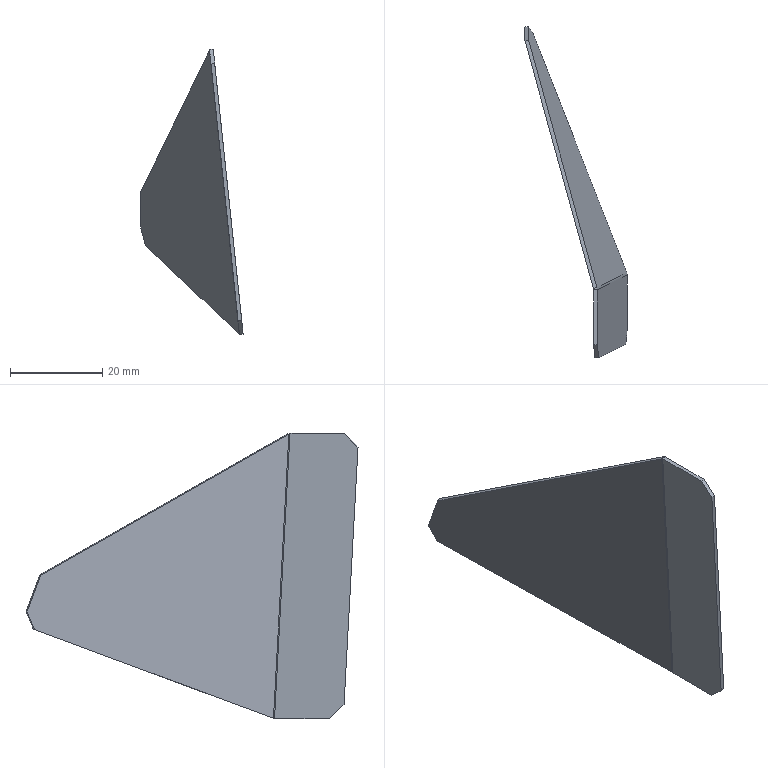Part | SolidWorks | features BaseBody 1 | 1 solid | 19 faces | box 22.146 x 71.822 x 61.748 mm | volume 2390 mm3 | plane 13 | spline 4 | cylinder 2 | commonest cylinder face diameters 1.473 x1 3.073 x1
STEP:
#1=CARTESIAN_POINT('',(255.936,161.31,493.18));
#2=VERTEX_POINT('',#1);
#3=CARTESIAN_POINT('',(262.393,164.643,431.747));
#4=VERTEX_POINT('',#3);
#5=CARTESIAN_POINT('',(255.882,161.282,493.701));
#6=DIRECTION('',(0.1044,0.05388,-0.9931));
#7=VECTOR('',#6,1000.);
#8=LINE('',#5,#7);
#9=EDGE_CURVE('',#2,#4,#8,.T.);
#10=ORIENTED_EDGE('',*,*,#9,.F.);
#11=CARTESIAN_POINT('',(241.126,214.983,462.654));
#12=VERTEX_POINT('',#11);
#13=CARTESIAN_POINT('',(241.126,214.983,462.654));
#14=DIRECTION('',(0.2332,-0.8453,0.4807));
#15=VECTOR('',#14,1000.);
#16=LINE('',#13,#15);
#17=EDGE_CURVE('',#12,#2,#16,.T.);
#18=ORIENTED_EDGE('',*,*,#17,.F.);
#19=CARTESIAN_POINT('',(241.093,217.909,454.745));
#20=VERTEX_POINT('',#19);
#21=CARTESIAN_POINT('',(241.093,217.909,454.745));
#22=DIRECTION('',(0.004002,-0.347,0.9379));
#23=VECTOR('',#22,1000.);
#24=LINE('',#21,#23);
#25=EDGE_CURVE('',#20,#12,#24,.T.);
#26=ORIENTED_EDGE('',*,*,#25,.F.);
#27=CARTESIAN_POINT('',(242.116,216.311,450.951));
#28=VERTEX_POINT('',#27);
#29=CARTESIAN_POINT('',(242.116,216.311,450.951));
#30=DIRECTION('',(-0.2413,0.3767,0.8944));
#31=VECTOR('',#30,1000.);
#32=LINE('',#29,#31);
#33=EDGE_CURVE('',#28,#20,#32,.T.);
#34=ORIENTED_EDGE('',*,*,#33,.F.);
#35=CARTESIAN_POINT('',(262.393,164.643,431.747));
#36=DIRECTION('',(-0.3452,0.8797,0.327));
#37=VECTOR('',#36,1000.);
#38=LINE('',#35,#37);
#39=EDGE_CURVE('',#4,#28,#38,.T.);
#40=ORIENTED_EDGE('',*,*,#39,.F.);
#41=EDGE_LOOP('',(#10,#18,#26,#34,#40));
#42=FACE_OUTER_BOUND('',#41,.T.);
#43=CARTESIAN_POINT('',(255.936,161.31,493.18));
#44=DIRECTION('',(0.9385,0.3251,0.1163));
#45=DIRECTION('',(0.122,0.002931,-0.9925));
#46=AXIS2_PLACEMENT_3D('',#43,#44,#45);
#47=PLANE('',#46);
#48=ADVANCED_FACE('',(#42),#47,.F.);
#49=CARTESIAN_POINT('',(242.867,216.571,451.044));
#50=VERTEX_POINT('',#49);
#51=CARTESIAN_POINT('',(242.492,216.441,450.997));
#52=DIRECTION('',(0.9385,0.3251,0.1163));
#53=VECTOR('',#52,1000.);
#54=LINE('',#51,#53);
#55=EDGE_CURVE('',#28,#50,#54,.T.);
#56=ORIENTED_EDGE('',*,*,#55,.T.);
#57=CARTESIAN_POINT('',(263.144,164.903,431.84));
#58=VERTEX_POINT('',#57);
#59=CARTESIAN_POINT('',(253.006,190.737,441.442));
#60=DIRECTION('',(0.3452,-0.8797,-0.327));
#61=VECTOR('',#60,1000.);
#62=LINE('',#59,#61);
#63=EDGE_CURVE('',#50,#58,#62,.T.);
#64=ORIENTED_EDGE('',*,*,#63,.T.);
#65=CARTESIAN_POINT('',(262.769,164.773,431.794));
#66=DIRECTION('',(-0.9385,-0.3251,-0.1163));
#67=VECTOR('',#66,1000.);
#68=LINE('',#65,#67);
#69=EDGE_CURVE('',#58,#4,#68,.T.);
#70=ORIENTED_EDGE('',*,*,#69,.T.);
#71=ORIENTED_EDGE('',*,*,#39,.T.);
#72=EDGE_LOOP('',(#56,#64,#70,#71));
#73=FACE_OUTER_BOUND('',#72,.T.);
#74=CARTESIAN_POINT('',(262.393,164.643,431.747));
#75=DIRECTION('',(-0.004002,0.347,-0.9379));
#76=DIRECTION('',(-0.3452,0.8797,0.327));
#77=AXIS2_PLACEMENT_3D('',#74,#75,#76);
#78=PLANE('',#77);
#79=ADVANCED_FACE('',(#73),#78,.T.);
#80=CARTESIAN_POINT('',(262.439,164.488,431.659));
#81=VERTEX_POINT('',#80);
#82=CARTESIAN_POINT('',(262.443,164.408,431.662));
#83=VERTEX_POINT('',#82);
#84=CARTESIAN_POINT('',(262.439,164.488,431.659));
#85=CARTESIAN_POINT('',(262.441,164.461,431.66));
#86=CARTESIAN_POINT('',(262.443,164.434,431.661));
#87=CARTESIAN_POINT('',(262.443,164.408,431.662));
#88=B_SPLINE_CURVE_WITH_KNOTS('',3,(#84,#85,#86,#87),.UNSPECIFIED.,.F.,.F.,(4,4),(0.,1.),.UNSPECIFIED.);
#89=EDGE_CURVE('',#81,#83,#88,.T.);
#90=ORIENTED_EDGE('',*,*,#89,.T.);
#91=CARTESIAN_POINT('',(255.962,161.062,493.323));
#92=VERTEX_POINT('',#91);
#93=CARTESIAN_POINT('',(259.203,162.735,462.489));
#94=DIRECTION('',(-0.1044,-0.05388,0.9931));
#95=VECTOR('',#94,1000.);
#96=LINE('',#93,#95);
#97=EDGE_CURVE('',#83,#92,#96,.T.);
#98=ORIENTED_EDGE('',*,*,#97,.T.);
#99=CARTESIAN_POINT('',(255.958,161.142,493.32));
#100=VERTEX_POINT('',#99);
#101=CARTESIAN_POINT('',(255.962,161.062,493.323));
#102=CARTESIAN_POINT('',(255.962,161.089,493.322));
#103=CARTESIAN_POINT('',(255.961,161.116,493.321));
#104=CARTESIAN_POINT('',(255.958,161.142,493.32));
#105=B_SPLINE_CURVE_WITH_KNOTS('',3,(#101,#102,#103,#104),.UNSPECIFIED.,.F.,.F.,(4,4),(0.,1.),.UNSPECIFIED.);
#106=EDGE_CURVE('',#92,#100,#105,.T.);
#107=ORIENTED_EDGE('',*,*,#106,.T.);
#108=CARTESIAN_POINT('',(255.958,161.142,493.32));
#109=CARTESIAN_POINT('',(255.957,161.199,493.274));
#110=CARTESIAN_POINT('',(255.949,161.256,493.227));
#111=CARTESIAN_POINT('',(255.936,161.31,493.18));
#112=B_SPLINE_CURVE_WITH_KNOTS('',3,(#108,#109,#110,#111),.UNSPECIFIED.,.F.,.F.,(4,4),(0.,1.),.UNSPECIFIED.);
#113=EDGE_CURVE('',#100,#2,#112,.T.);
#114=ORIENTED_EDGE('',*,*,#113,.T.);
#115=ORIENTED_EDGE('',*,*,#9,.T.);
#116=CARTESIAN_POINT('',(262.393,164.643,431.747));
#117=CARTESIAN_POINT('',(262.414,164.593,431.719));
#118=CARTESIAN_POINT('',(262.429,164.541,431.689));
#119=CARTESIAN_POINT('',(262.439,164.488,431.659));
#120=B_SPLINE_CURVE_WITH_KNOTS('',3,(#116,#117,#118,#119),.UNSPECIFIED.,.F.,.F.,(4,4),(0.,1.),.UNSPECIFIED.);
#121=EDGE_CURVE('',#4,#81,#120,.T.);
#122=ORIENTED_EDGE('',*,*,#121,.T.);
#123=EDGE_LOOP('',(#90,#98,#107,#114,#115,#122));
#124=FACE_OUTER_BOUND('',#123,.T.);
#125=CARTESIAN_POINT('',(255.19,161.042,493.616));
#126=DIRECTION('',(0.1044,0.05388,-0.9931));
#127=DIRECTION('',(-0.9945,0.,-0.1045));
#128=AXIS2_PLACEMENT_3D('',#125,#126,#127);
#129=CYLINDRICAL_SURFACE('',#128,0.7366);
#130=ADVANCED_FACE('',(#124),#129,.F.);
#131=CARTESIAN_POINT('',(241.877,215.243,462.747));
#132=VERTEX_POINT('',#131);
#133=CARTESIAN_POINT('',(241.502,215.113,462.7));
#134=DIRECTION('',(-0.9385,-0.3251,-0.1163));
#135=VECTOR('',#134,1000.);
#136=LINE('',#133,#135);
#137=EDGE_CURVE('',#132,#12,#136,.T.);
#138=ORIENTED_EDGE('',*,*,#137,.T.);
#139=ORIENTED_EDGE('',*,*,#17,.T.);
#140=CARTESIAN_POINT('',(256.687,161.57,493.273));
#141=VERTEX_POINT('',#140);
#142=CARTESIAN_POINT('',(256.312,161.44,493.226));
#143=DIRECTION('',(0.9385,0.3251,0.1163));
#144=VECTOR('',#143,1000.);
#145=LINE('',#142,#144);
#146=EDGE_CURVE('',#2,#141,#145,.T.);
#147=ORIENTED_EDGE('',*,*,#146,.T.);
#148=CARTESIAN_POINT('',(249.282,188.407,478.01));
#149=DIRECTION('',(-0.2332,0.8453,-0.4807));
#150=VECTOR('',#149,1000.);
#151=LINE('',#148,#150);
#152=EDGE_CURVE('',#141,#132,#151,.T.);
#153=ORIENTED_EDGE('',*,*,#152,.T.);
#154=EDGE_LOOP('',(#138,#139,#147,#153));
#155=FACE_OUTER_BOUND('',#154,.T.);
#156=CARTESIAN_POINT('',(241.126,214.983,462.654));
#157=DIRECTION('',(-0.2546,0.4241,0.8691));
#158=DIRECTION('',(0.2332,-0.8453,0.4807));
#159=AXIS2_PLACEMENT_3D('',#156,#157,#158);
#160=PLANE('',#159);
#161=ADVANCED_FACE('',(#155),#160,.T.);
#162=ORIENTED_EDGE('',*,*,#25,.T.);
#163=ORIENTED_EDGE('',*,*,#137,.F.);
#164=CARTESIAN_POINT('',(241.843,218.17,454.838));
#165=VERTEX_POINT('',#164);
#166=CARTESIAN_POINT('',(241.86,216.706,458.793));
#167=DIRECTION('',(-0.004002,0.347,-0.9379));
#168=VECTOR('',#167,1000.);
#169=LINE('',#166,#168);
#170=EDGE_CURVE('',#132,#165,#169,.T.);
#171=ORIENTED_EDGE('',*,*,#170,.T.);
#172=CARTESIAN_POINT('',(241.468,218.04,454.792));
#173=DIRECTION('',(-0.9385,-0.3251,-0.1163));
#174=VECTOR('',#173,1000.);
#175=LINE('',#172,#174);
#176=EDGE_CURVE('',#165,#20,#175,.T.);
#177=ORIENTED_EDGE('',*,*,#176,.T.);
#178=EDGE_LOOP('',(#162,#163,#171,#177));
#179=FACE_OUTER_BOUND('',#178,.T.);
#180=CARTESIAN_POINT('',(241.093,217.909,454.745));
#181=DIRECTION('',(-0.3452,0.8797,0.327));
#182=DIRECTION('',(0.004002,-0.347,0.9379));
#183=AXIS2_PLACEMENT_3D('',#180,#181,#182);
#184=PLANE('',#183);
#185=ADVANCED_FACE('',(#179),#184,.T.);
#186=ORIENTED_EDGE('',*,*,#33,.T.);
#187=ORIENTED_EDGE('',*,*,#176,.F.);
#188=CARTESIAN_POINT('',(242.355,217.37,452.941));
#189=DIRECTION('',(0.2413,-0.3767,-0.8944));
#190=VECTOR('',#189,1000.);
#191=LINE('',#188,#190);
#192=EDGE_CURVE('',#165,#50,#191,.T.);
#193=ORIENTED_EDGE('',*,*,#192,.T.);
#194=ORIENTED_EDGE('',*,*,#55,.F.);
#195=EDGE_LOOP('',(#186,#187,#193,#194));
#196=FACE_OUTER_BOUND('',#195,.T.);
#197=CARTESIAN_POINT('',(242.116,216.311,450.951));
#198=DIRECTION('',(-0.247,0.8674,-0.432));
#199=DIRECTION('',(-0.2413,0.3767,0.8944));
#200=AXIS2_PLACEMENT_3D('',#197,#198,#199);
#201=PLANE('',#200);
#202=ADVANCED_FACE('',(#196),#201,.T.);
#203=ORIENTED_EDGE('',*,*,#170,.F.);
#204=ORIENTED_EDGE('',*,*,#152,.F.);
#205=CARTESIAN_POINT('',(256.687,161.57,493.273));
#206=DIRECTION('',(0.1044,0.05388,-0.9931));
#207=VECTOR('',#206,1000.);
#208=LINE('',#205,#207);
#209=EDGE_CURVE('',#141,#58,#208,.T.);
#210=ORIENTED_EDGE('',*,*,#209,.T.);
#211=ORIENTED_EDGE('',*,*,#63,.F.);
#212=ORIENTED_EDGE('',*,*,#192,.F.);
#213=EDGE_LOOP('',(#203,#204,#210,#211,#212));
#214=FACE_OUTER_BOUND('',#213,.T.);
#215=CARTESIAN_POINT('',(256.687,161.57,493.273));
#216=DIRECTION('',(0.9385,0.3251,0.1163));
#217=DIRECTION('',(0.122,0.002931,-0.9925));
#218=AXIS2_PLACEMENT_3D('',#215,#216,#217);
#219=PLANE('',#218);
#220=ADVANCED_FACE('',(#214),#219,.T.);
#221=CARTESIAN_POINT('',(263.229,164.574,431.747));
#222=VERTEX_POINT('',#221);
#223=CARTESIAN_POINT('',(263.229,164.574,431.747));
#224=CARTESIAN_POINT('',(263.213,164.686,431.78));
#225=CARTESIAN_POINT('',(263.185,164.797,431.811));
#226=CARTESIAN_POINT('',(263.144,164.903,431.84));
#227=B_SPLINE_CURVE_WITH_KNOTS('',3,(#223,#224,#225,#226),.UNSPECIFIED.,.F.,.F.,(4,4),(0.,1.),.UNSPECIFIED.);
#228=EDGE_CURVE('',#222,#58,#227,.T.);
#229=ORIENTED_EDGE('',*,*,#228,.F.);
#230=CARTESIAN_POINT('',(262.834,164.531,431.703));
#231=DIRECTION('',(0.9881,0.1081,0.1097));
#232=VECTOR('',#231,1000.);
#233=LINE('',#230,#232);
#234=EDGE_CURVE('',#81,#222,#233,.T.);
#235=ORIENTED_EDGE('',*,*,#234,.F.);
#236=ORIENTED_EDGE('',*,*,#121,.F.);
#237=ORIENTED_EDGE('',*,*,#69,.F.);
#238=EDGE_LOOP('',(#229,#235,#236,#237));
#239=FACE_OUTER_BOUND('',#238,.T.);
#240=CARTESIAN_POINT('',(263.144,164.903,431.84));
#241=CARTESIAN_POINT('',(263.185,164.797,431.811));
#242=CARTESIAN_POINT('',(263.213,164.686,431.78));
#243=CARTESIAN_POINT('',(263.229,164.574,431.747));
#244=CARTESIAN_POINT('',(262.393,164.643,431.747));
#245=CARTESIAN_POINT('',(262.414,164.593,431.719));
#246=CARTESIAN_POINT('',(262.429,164.541,431.689));
#247=CARTESIAN_POINT('',(262.439,164.488,431.659));
#248=B_SPLINE_SURFACE_WITH_KNOTS('',1,3,((#240,#241,#242,#243),(#244,#245,#246,#247)),.UNSPECIFIED.,.F.,.F.,.F.,(2,2),(4,4),(0.,1.),(0.,1.),.UNSPECIFIED.);
#249=ADVANCED_FACE('',(#239),#248,.F.);
#250=CARTESIAN_POINT('',(262.443,152.531,431.662));
#251=VERTEX_POINT('',#250);
#252=CARTESIAN_POINT('',(262.443,155.378,431.662));
#253=DIRECTION('',(0.,1.,0.));
#254=VECTOR('',#253,1000.);
#255=LINE('',#252,#254);
#256=EDGE_CURVE('',#251,#83,#255,.T.);
#257=ORIENTED_EDGE('',*,*,#256,.F.);
#258=CARTESIAN_POINT('',(262.129,149.369,434.641));
#259=VERTEX_POINT('',#258);
#260=CARTESIAN_POINT('',(262.129,149.369,434.641));
#261=DIRECTION('',(0.07189,0.7259,-0.684));
#262=VECTOR('',#261,1000.);
#263=LINE('',#260,#262);
#264=EDGE_CURVE('',#259,#251,#263,.T.);
#265=ORIENTED_EDGE('',*,*,#264,.F.);
#266=CARTESIAN_POINT('',(256.275,146.347,490.343));
#267=VERTEX_POINT('',#266);
#268=CARTESIAN_POINT('',(256.275,146.347,490.343));
#269=DIRECTION('',(0.1044,0.05388,-0.9931));
#270=VECTOR('',#269,1000.);
#271=LINE('',#268,#270);
#272=EDGE_CURVE('',#267,#259,#271,.T.);
#273=ORIENTED_EDGE('',*,*,#272,.F.);
#274=CARTESIAN_POINT('',(255.962,149.186,493.323));
#275=VERTEX_POINT('',#274);
#276=CARTESIAN_POINT('',(255.962,149.186,493.323));
#277=DIRECTION('',(0.07588,-0.6878,-0.7219));
#278=VECTOR('',#277,1000.);
#279=LINE('',#276,#278);
#280=EDGE_CURVE('',#275,#267,#279,.T.);
#281=ORIENTED_EDGE('',*,*,#280,.F.);
#282=CARTESIAN_POINT('',(255.962,155.378,493.323));
#283=DIRECTION('',(0.,-1.,0.));
#284=VECTOR('',#283,1000.);
#285=LINE('',#282,#284);
#286=EDGE_CURVE('',#92,#275,#285,.T.);
#287=ORIENTED_EDGE('',*,*,#286,.F.);
#288=ORIENTED_EDGE('',*,*,#97,.F.);
#289=EDGE_LOOP('',(#257,#265,#273,#281,#287,#288));
#290=FACE_OUTER_BOUND('',#289,.T.);
#291=CARTESIAN_POINT('',(255.962,146.347,493.323));
#292=DIRECTION('',(0.9945,0.,0.1045));
#293=DIRECTION('',(0.1045,0.,-0.9945));
#294=AXIS2_PLACEMENT_3D('',#291,#292,#293);
#295=PLANE('',#294);
#296=ADVANCED_FACE('',(#290),#295,.F.);
#297=CARTESIAN_POINT('',(263.238,164.408,431.746));
#298=VERTEX_POINT('',#297);
#299=CARTESIAN_POINT('',(263.238,164.408,431.746));
#300=CARTESIAN_POINT('',(263.238,164.463,431.747));
#301=CARTESIAN_POINT('',(263.235,164.519,431.747));
#302=CARTESIAN_POINT('',(263.229,164.574,431.747));
#303=B_SPLINE_CURVE_WITH_KNOTS('',3,(#299,#300,#301,#302),.UNSPECIFIED.,.F.,.F.,(4,4),(0.,1.),.UNSPECIFIED.);
#304=EDGE_CURVE('',#298,#222,#303,.T.);
#305=ORIENTED_EDGE('',*,*,#304,.F.);
#306=CARTESIAN_POINT('',(262.84,164.408,431.704));
#307=DIRECTION('',(0.9945,0.,0.1045));
#308=VECTOR('',#307,1000.);
#309=LINE('',#306,#308);
#310=EDGE_CURVE('',#83,#298,#309,.T.);
#311=ORIENTED_EDGE('',*,*,#310,.F.);
#312=ORIENTED_EDGE('',*,*,#89,.F.);
#313=ORIENTED_EDGE('',*,*,#234,.T.);
#314=EDGE_LOOP('',(#305,#311,#312,#313));
#315=FACE_OUTER_BOUND('',#314,.T.);
#316=CARTESIAN_POINT('',(263.229,164.574,431.747));
#317=CARTESIAN_POINT('',(263.235,164.519,431.747));
#318=CARTESIAN_POINT('',(263.238,164.463,431.747));
#319=CARTESIAN_POINT('',(263.238,164.408,431.746));
#320=CARTESIAN_POINT('',(262.439,164.488,431.659));
#321=CARTESIAN_POINT('',(262.441,164.461,431.66));
#322=CARTESIAN_POINT('',(262.443,164.434,431.661));
#323=CARTESIAN_POINT('',(262.443,164.408,431.662));
#324=B_SPLINE_SURFACE_WITH_KNOTS('',1,3,((#316,#317,#318,#319),(#320,#321,#322,#323)),.UNSPECIFIED.,.F.,.F.,.F.,(2,2),(4,4),(0.,1.),(0.,1.),.UNSPECIFIED.);
#325=ADVANCED_FACE('',(#315),#324,.F.);
#326=ORIENTED_EDGE('',*,*,#146,.F.);
#327=ORIENTED_EDGE('',*,*,#113,.F.);
#328=CARTESIAN_POINT('',(256.748,161.229,493.408));
#329=VERTEX_POINT('',#328);
#330=CARTESIAN_POINT('',(256.353,161.186,493.364));
#331=DIRECTION('',(-0.9881,-0.1081,-0.1097));
#332=VECTOR('',#331,1000.);
#333=LINE('',#330,#332);
#334=EDGE_CURVE('',#329,#100,#333,.T.);
#335=ORIENTED_EDGE('',*,*,#334,.F.);
#336=CARTESIAN_POINT('',(256.687,161.57,493.273));
#337=CARTESIAN_POINT('',(256.72,161.46,493.319));
#338=CARTESIAN_POINT('',(256.74,161.345,493.364));
#339=CARTESIAN_POINT('',(256.748,161.229,493.408));
#340=B_SPLINE_CURVE_WITH_KNOTS('',3,(#336,#337,#338,#339),.UNSPECIFIED.,.F.,.F.,(4,4),(0.,1.),.UNSPECIFIED.);
#341=EDGE_CURVE('',#141,#329,#340,.T.);
#342=ORIENTED_EDGE('',*,*,#341,.F.);
#343=EDGE_LOOP('',(#326,#327,#335,#342));
#344=FACE_OUTER_BOUND('',#343,.T.);
#345=CARTESIAN_POINT('',(256.748,161.229,493.408));
#346=CARTESIAN_POINT('',(256.74,161.345,493.364));
#347=CARTESIAN_POINT('',(256.72,161.46,493.319));
#348=CARTESIAN_POINT('',(256.687,161.57,493.273));
#349=CARTESIAN_POINT('',(255.958,161.142,493.32));
#350=CARTESIAN_POINT('',(255.957,161.199,493.274));
#351=CARTESIAN_POINT('',(255.949,161.256,493.227));
#352=CARTESIAN_POINT('',(255.936,161.31,493.18));
#353=B_SPLINE_SURFACE_WITH_KNOTS('',1,3,((#345,#346,#347,#348),(#349,#350,#351,#352)),.UNSPECIFIED.,.F.,.F.,.F.,(2,2),(4,4),(0.,1.),(0.,1.),.UNSPECIFIED.);
#354=ADVANCED_FACE('',(#344),#353,.F.);
#355=CARTESIAN_POINT('',(256.757,161.062,493.406));
#356=VERTEX_POINT('',#355);
#357=CARTESIAN_POINT('',(256.748,161.229,493.408));
#358=CARTESIAN_POINT('',(256.754,161.173,493.407));
#359=CARTESIAN_POINT('',(256.757,161.118,493.407));
#360=CARTESIAN_POINT('',(256.757,161.062,493.406));
#361=B_SPLINE_CURVE_WITH_KNOTS('',3,(#357,#358,#359,#360),.UNSPECIFIED.,.F.,.F.,(4,4),(0.000003891,1.),.UNSPECIFIED.);
#362=EDGE_CURVE('',#329,#356,#361,.T.);
#363=ORIENTED_EDGE('',*,*,#362,.F.);
#364=ORIENTED_EDGE('',*,*,#334,.T.);
#365=ORIENTED_EDGE('',*,*,#106,.F.);
#366=CARTESIAN_POINT('',(256.36,161.062,493.364));
#367=DIRECTION('',(-0.9945,0.,-0.1045));
#368=VECTOR('',#367,1000.);
#369=LINE('',#366,#368);
#370=EDGE_CURVE('',#356,#92,#369,.T.);
#371=ORIENTED_EDGE('',*,*,#370,.F.);
#372=EDGE_LOOP('',(#363,#364,#365,#371));
#373=FACE_OUTER_BOUND('',#372,.T.);
#374=CARTESIAN_POINT('',(256.757,161.062,493.406));
#375=CARTESIAN_POINT('',(256.757,161.118,493.407));
#376=CARTESIAN_POINT('',(256.754,161.173,493.407));
#377=CARTESIAN_POINT('',(256.748,161.229,493.408));
#378=CARTESIAN_POINT('',(255.962,161.062,493.323));
#379=CARTESIAN_POINT('',(255.962,161.089,493.322));
#380=CARTESIAN_POINT('',(255.961,161.116,493.321));
#381=CARTESIAN_POINT('',(255.958,161.142,493.32));
#382=B_SPLINE_SURFACE_WITH_KNOTS('',1,3,((#374,#375,#376,#377),(#378,#379,#380,#381)),.UNSPECIFIED.,.F.,.F.,.F.,(2,2),(4,4),(0.,1.),(0.,1.),.UNSPECIFIED.);
#383=ADVANCED_FACE('',(#373),#382,.F.);
#384=CARTESIAN_POINT('',(259.998,162.735,462.573));
#385=DIRECTION('',(-0.1044,-0.05388,0.9931));
#386=VECTOR('',#385,1000.);
#387=LINE('',#384,#386);
#388=EDGE_CURVE('',#298,#356,#387,.T.);
#389=ORIENTED_EDGE('',*,*,#388,.F.);
#390=ORIENTED_EDGE('',*,*,#304,.T.);
#391=ORIENTED_EDGE('',*,*,#228,.T.);
#392=ORIENTED_EDGE('',*,*,#209,.F.);
#393=ORIENTED_EDGE('',*,*,#341,.T.);
#394=ORIENTED_EDGE('',*,*,#362,.T.);
#395=EDGE_LOOP('',(#389,#390,#391,#392,#393,#394));
#396=FACE_OUTER_BOUND('',#395,.T.);
#397=CARTESIAN_POINT('',(255.19,161.042,493.616));
#398=DIRECTION('',(0.1044,0.05388,-0.9931));
#399=DIRECTION('',(-0.9945,0.,-0.1045));
#400=AXIS2_PLACEMENT_3D('',#397,#398,#399);
#401=CYLINDRICAL_SURFACE('',#400,1.537);
#402=ADVANCED_FACE('',(#396),#401,.T.);
#403=CARTESIAN_POINT('',(263.238,152.531,431.746));
#404=VERTEX_POINT('',#403);
#405=CARTESIAN_POINT('',(263.238,158.469,431.746));
#406=DIRECTION('',(0.,-1.,0.));
#407=VECTOR('',#406,1000.);
#408=LINE('',#405,#407);
#409=EDGE_CURVE('',#298,#404,#408,.T.);
#410=ORIENTED_EDGE('',*,*,#409,.T.);
#411=CARTESIAN_POINT('',(262.84,152.531,431.704));
#412=DIRECTION('',(-0.9945,0.,-0.1045));
#413=VECTOR('',#412,1000.);
#414=LINE('',#411,#413);
#415=EDGE_CURVE('',#404,#251,#414,.T.);
#416=ORIENTED_EDGE('',*,*,#415,.T.);
#417=ORIENTED_EDGE('',*,*,#256,.T.);
#418=ORIENTED_EDGE('',*,*,#310,.T.);
#419=EDGE_LOOP('',(#410,#416,#417,#418));
#420=FACE_OUTER_BOUND('',#419,.T.);
#421=CARTESIAN_POINT('',(262.443,152.531,431.662));
#422=DIRECTION('',(0.1045,0.,-0.9945));
#423=DIRECTION('',(0.,1.,0.));
#424=AXIS2_PLACEMENT_3D('',#421,#422,#423);
#425=PLANE('',#424);
#426=ADVANCED_FACE('',(#420),#425,.T.);
#427=ORIENTED_EDGE('',*,*,#264,.T.);
#428=ORIENTED_EDGE('',*,*,#415,.F.);
#429=CARTESIAN_POINT('',(262.925,149.369,434.725));
#430=VERTEX_POINT('',#429);
#431=CARTESIAN_POINT('',(263.082,150.95,433.235));
#432=DIRECTION('',(-0.07189,-0.7259,0.684));
#433=VECTOR('',#432,1000.);
#434=LINE('',#431,#433);
#435=EDGE_CURVE('',#404,#430,#434,.T.);
#436=ORIENTED_EDGE('',*,*,#435,.T.);
#437=CARTESIAN_POINT('',(262.527,149.369,434.683));
#438=DIRECTION('',(-0.9945,0.,-0.1045));
#439=VECTOR('',#438,1000.);
#440=LINE('',#437,#439);
#441=EDGE_CURVE('',#430,#259,#440,.T.);
#442=ORIENTED_EDGE('',*,*,#441,.T.);
#443=EDGE_LOOP('',(#427,#428,#436,#442));
#444=FACE_OUTER_BOUND('',#443,.T.);
#445=CARTESIAN_POINT('',(262.129,149.369,434.641));
#446=DIRECTION('',(0.07588,-0.6878,-0.7219));
#447=DIRECTION('',(0.07189,0.7259,-0.684));
#448=AXIS2_PLACEMENT_3D('',#445,#446,#447);
#449=PLANE('',#448);
#450=ADVANCED_FACE('',(#444),#449,.T.);
#451=ORIENTED_EDGE('',*,*,#272,.T.);
#452=ORIENTED_EDGE('',*,*,#441,.F.);
#453=CARTESIAN_POINT('',(257.071,146.347,490.427));
#454=VERTEX_POINT('',#453);
#455=CARTESIAN_POINT('',(259.998,147.858,462.576));
#456=DIRECTION('',(-0.1044,-0.05388,0.9931));
#457=VECTOR('',#456,1000.);
#458=LINE('',#455,#457);
#459=EDGE_CURVE('',#430,#454,#458,.T.);
#460=ORIENTED_EDGE('',*,*,#459,.T.);
#461=CARTESIAN_POINT('',(256.673,146.347,490.385));
#462=DIRECTION('',(-0.9945,0.,-0.1045));
#463=VECTOR('',#462,1000.);
#464=LINE('',#461,#463);
#465=EDGE_CURVE('',#454,#267,#464,.T.);
#466=ORIENTED_EDGE('',*,*,#465,.T.);
#467=EDGE_LOOP('',(#451,#452,#460,#466));
#468=FACE_OUTER_BOUND('',#467,.T.);
#469=CARTESIAN_POINT('',(256.275,146.347,490.343));
#470=DIRECTION('',(0.005632,-0.9985,-0.05358));
#471=DIRECTION('',(0.1044,0.05388,-0.9931));
#472=AXIS2_PLACEMENT_3D('',#469,#470,#471);
#473=PLANE('',#472);
#474=ADVANCED_FACE('',(#468),#473,.T.);
#475=ORIENTED_EDGE('',*,*,#280,.T.);
#476=ORIENTED_EDGE('',*,*,#465,.F.);
#477=CARTESIAN_POINT('',(256.757,149.186,493.406));
#478=VERTEX_POINT('',#477);
#479=CARTESIAN_POINT('',(256.914,147.767,491.917));
#480=DIRECTION('',(-0.07588,0.6878,0.7219));
#481=VECTOR('',#480,1000.);
#482=LINE('',#479,#481);
#483=EDGE_CURVE('',#454,#478,#482,.T.);
#484=ORIENTED_EDGE('',*,*,#483,.T.);
#485=CARTESIAN_POINT('',(256.36,149.186,493.364));
#486=DIRECTION('',(-0.9945,0.,-0.1045));
#487=VECTOR('',#486,1000.);
#488=LINE('',#485,#487);
#489=EDGE_CURVE('',#478,#275,#488,.T.);
#490=ORIENTED_EDGE('',*,*,#489,.T.);
#491=EDGE_LOOP('',(#475,#476,#484,#490));
#492=FACE_OUTER_BOUND('',#491,.T.);
#493=CARTESIAN_POINT('',(255.962,149.186,493.323));
#494=DIRECTION('',(-0.07189,-0.7259,0.684));
#495=DIRECTION('',(0.07588,-0.6878,-0.7219));
#496=AXIS2_PLACEMENT_3D('',#493,#494,#495);
#497=PLANE('',#496);
#498=ADVANCED_FACE('',(#492),#497,.T.);
#499=ORIENTED_EDGE('',*,*,#286,.T.);
#500=ORIENTED_EDGE('',*,*,#489,.F.);
#501=CARTESIAN_POINT('',(256.757,155.124,493.406));
#502=DIRECTION('',(0.,1.,0.));
#503=VECTOR('',#502,1000.);
#504=LINE('',#501,#503);
#505=EDGE_CURVE('',#478,#356,#504,.T.);
#506=ORIENTED_EDGE('',*,*,#505,.T.);
#507=ORIENTED_EDGE('',*,*,#370,.T.);
#508=EDGE_LOOP('',(#499,#500,#506,#507));
#509=FACE_OUTER_BOUND('',#508,.T.);
#510=CARTESIAN_POINT('',(255.962,161.062,493.323));
#511=DIRECTION('',(-0.1045,0.,0.9945));
#512=DIRECTION('',(0.,-1.,0.));
#513=AXIS2_PLACEMENT_3D('',#510,#511,#512);
#514=PLANE('',#513);
#515=ADVANCED_FACE('',(#509),#514,.T.);
#516=ORIENTED_EDGE('',*,*,#459,.F.);
#517=ORIENTED_EDGE('',*,*,#435,.F.);
#518=ORIENTED_EDGE('',*,*,#409,.F.);
#519=ORIENTED_EDGE('',*,*,#388,.T.);
#520=ORIENTED_EDGE('',*,*,#505,.F.);
#521=ORIENTED_EDGE('',*,*,#483,.F.);
#522=EDGE_LOOP('',(#516,#517,#518,#519,#520,#521));
#523=FACE_OUTER_BOUND('',#522,.T.);
#524=CARTESIAN_POINT('',(256.757,146.347,493.406));
#525=DIRECTION('',(0.9945,0.,0.1045));
#526=DIRECTION('',(0.1045,0.,-0.9945));
#527=AXIS2_PLACEMENT_3D('',#524,#525,#526);
#528=PLANE('',#527);
#529=ADVANCED_FACE('',(#523),#528,.T.);
#530=CLOSED_SHELL('',(#48,#79,#130,#161,#185,#202,#220,#249,#296,#325,#354,#383,#402,#426,#450,#474,#498,#515,#529));
#531=MANIFOLD_SOLID_BREP('',#530);
#532=CARTESIAN_POINT('',(0.,0.,0.));
#533=DIRECTION('',(0.,0.,1.));
#534=DIRECTION('',(1.,0.,0.));
#535=AXIS2_PLACEMENT_3D('',#532,#533,#534);
#536=(LENGTH_UNIT()NAMED_UNIT(*)SI_UNIT(.MILLI.,.METRE.));
#537=UNCERTAINTY_MEASURE_WITH_UNIT(LENGTH_MEASURE(0.00001),#536,'','');
#538=(NAMED_UNIT(*)PLANE_ANGLE_UNIT()SI_UNIT($,.RADIAN.));
#539=(NAMED_UNIT(*)SI_UNIT($,.STERADIAN.)SOLID_ANGLE_UNIT());
#540=(GEOMETRIC_REPRESENTATION_CONTEXT(3)GLOBAL_UNCERTAINTY_ASSIGNED_CONTEXT((#537))GLOBAL_UNIT_ASSIGNED_CONTEXT((#536,#538,#539))REPRESENTATION_CONTEXT('',''));
#541=ADVANCED_BREP_SHAPE_REPRESENTATION('',(#531,#535),#540);